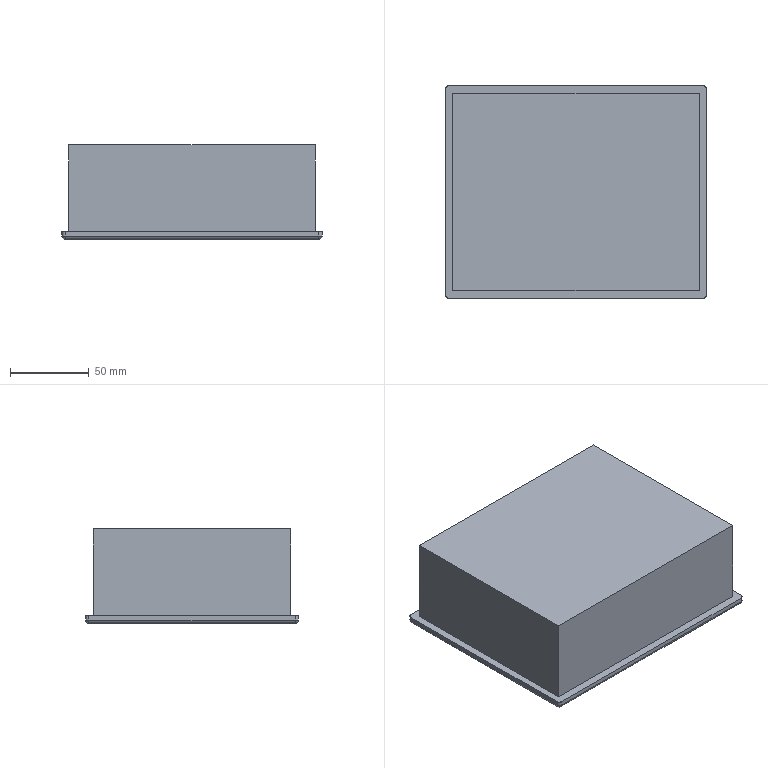Part | STEP file | Touch screen | 1 solid | 28 faces | box 165 x 135 x 59.8 mm | volume 1170552 mm3 | plane 12 | cylinder 12 | spline 4 | commonest cylinder face diameters 4 x12